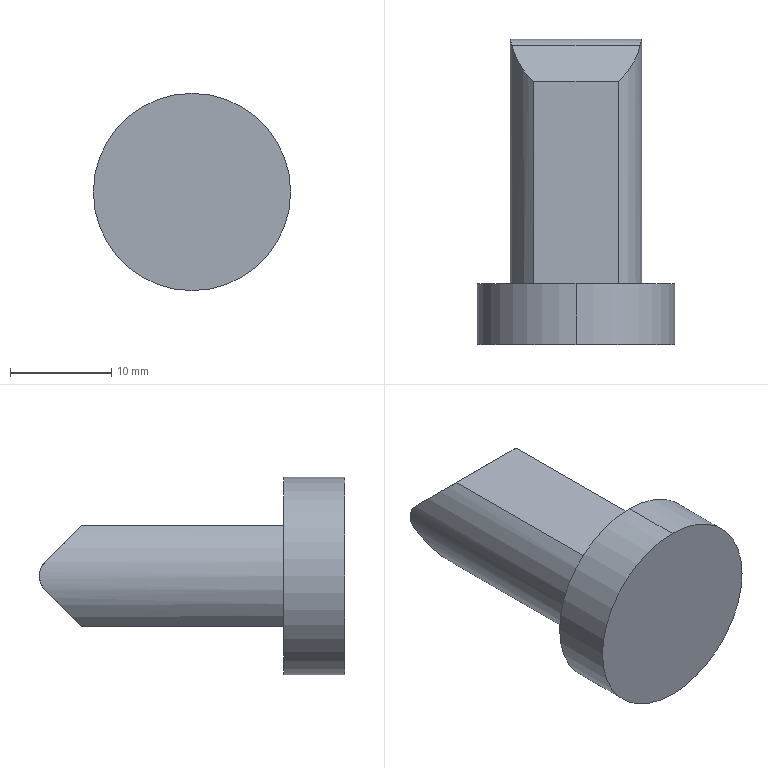Part | STEP file | Trava gavetas - Torre - 1 cav | 1 solid | 11 faces | box 19.5 x 30.172 x 19.5 mm | volume 4402 mm3 | plane 6 | cylinder 5 | commonest cylinder face diameters 13 x2 19.5 x2 4 x1
STEP:
#1=CARTESIAN_POINT('',(0.,0.,0.));
#2=DIRECTION('',(0.,0.,1.));
#3=DIRECTION('',(1.,0.,0.));
#4=AXIS2_PLACEMENT_3D('',#1,#2,#3);
#5=CARTESIAN_POINT('',(0.,0.,9.75));
#6=VERTEX_POINT('',#5);
#7=CARTESIAN_POINT('',(0.,0.,-9.75));
#8=VERTEX_POINT('',#7);
#9=CARTESIAN_POINT('',(0.,0.,0.));
#10=DIRECTION('',(0.,1.,0.));
#11=DIRECTION('',(0.,0.,1.));
#12=AXIS2_PLACEMENT_3D('',#9,#10,#11);
#13=CIRCLE('',#12,9.75);
#14=CARTESIAN_POINT('',(0.,31.,0.));
#15=DIRECTION('',(0.,1.,0.));
#16=DIRECTION('',(0.,0.,1.));
#17=AXIS2_PLACEMENT_3D('',#14,#15,#16);
#18=CYLINDRICAL_SURFACE('',#17,9.75);
#19=CARTESIAN_POINT('',(0.,-31.));
#20=DIRECTION('',(1.,0.));
#21=VECTOR('',#20,1.);
#22=LINE('',#19,#21);
#23=(GEOMETRIC_REPRESENTATION_CONTEXT(2)PARAMETRIC_REPRESENTATION_CONTEXT()REPRESENTATION_CONTEXT('',''));
#24=DEFINITIONAL_REPRESENTATION('',(#22),#23);
#25=PCURVE('',#18,#24);
#26=CARTESIAN_POINT('',(0.,0.,0.));
#27=DIRECTION('',(0.,1.,0.));
#28=DIRECTION('',(0.,0.,1.));
#29=AXIS2_PLACEMENT_3D('',#26,#27,#28);
#30=PLANE('',#29);
#31=CARTESIAN_POINT('',(0.,0.));
#32=DIRECTION('',(1.,0.));
#33=AXIS2_PLACEMENT_2D('',#31,#32);
#34=CIRCLE('',#33,9.75);
#35=(GEOMETRIC_REPRESENTATION_CONTEXT(2)PARAMETRIC_REPRESENTATION_CONTEXT()REPRESENTATION_CONTEXT('',''));
#36=DEFINITIONAL_REPRESENTATION('',(#34),#35);
#37=PCURVE('',#30,#36);
#38=SURFACE_CURVE('',#13,(#25,#37),.PCURVE_S1.);
#39=EDGE_CURVE('',#6,#8,#38,.T.);
#40=ORIENTED_EDGE('',*,*,#39,.T.);
#41=CARTESIAN_POINT('',(0.,6.,-9.75));
#42=VERTEX_POINT('',#41);
#43=CARTESIAN_POINT('',(0.,31.,-9.75));
#44=DIRECTION('',(0.,1.,0.));
#45=VECTOR('',#44,1.);
#46=LINE('',#43,#45);
#47=CARTESIAN_POINT('',(3.142,0.));
#48=DIRECTION('',(0.,1.));
#49=VECTOR('',#48,1.);
#50=LINE('',#47,#49);
#51=(GEOMETRIC_REPRESENTATION_CONTEXT(2)PARAMETRIC_REPRESENTATION_CONTEXT()REPRESENTATION_CONTEXT('',''));
#52=DEFINITIONAL_REPRESENTATION('',(#50),#51);
#53=PCURVE('',#18,#52);
#54=CARTESIAN_POINT('',(0.,31.,0.));
#55=DIRECTION('',(0.,1.,0.));
#56=DIRECTION('',(0.,0.,1.));
#57=AXIS2_PLACEMENT_3D('',#54,#55,#56);
#58=CYLINDRICAL_SURFACE('',#57,9.75);
#59=CARTESIAN_POINT('',(3.142,0.));
#60=DIRECTION('',(0.,1.));
#61=VECTOR('',#60,1.);
#62=LINE('',#59,#61);
#63=(GEOMETRIC_REPRESENTATION_CONTEXT(2)PARAMETRIC_REPRESENTATION_CONTEXT()REPRESENTATION_CONTEXT('',''));
#64=DEFINITIONAL_REPRESENTATION('',(#62),#63);
#65=PCURVE('',#58,#64);
#66=SURFACE_CURVE('',#46,(#53,#65),.PCURVE_S1.);
#67=EDGE_CURVE('',#8,#42,#66,.T.);
#68=ORIENTED_EDGE('',*,*,#67,.T.);
#69=CARTESIAN_POINT('',(0.,6.,9.75));
#70=VERTEX_POINT('',#69);
#71=CARTESIAN_POINT('',(0.,6.,0.));
#72=DIRECTION('',(0.,1.,0.));
#73=DIRECTION('',(0.,0.,1.));
#74=AXIS2_PLACEMENT_3D('',#71,#72,#73);
#75=CIRCLE('',#74,9.75);
#76=CARTESIAN_POINT('',(0.,-25.));
#77=DIRECTION('',(1.,0.));
#78=VECTOR('',#77,1.);
#79=LINE('',#76,#78);
#80=(GEOMETRIC_REPRESENTATION_CONTEXT(2)PARAMETRIC_REPRESENTATION_CONTEXT()REPRESENTATION_CONTEXT('',''));
#81=DEFINITIONAL_REPRESENTATION('',(#79),#80);
#82=PCURVE('',#18,#81);
#83=CARTESIAN_POINT('',(0.,6.,-9.75));
#84=DIRECTION('',(0.,-1.,0.));
#85=DIRECTION('',(0.,0.,-1.));
#86=AXIS2_PLACEMENT_3D('',#83,#84,#85);
#87=PLANE('',#86);
#88=CARTESIAN_POINT('',(-19.5,0.));
#89=CARTESIAN_POINT('',(-19.5,16.887));
#90=CARTESIAN_POINT('',(-4.875,8.444));
#91=CARTESIAN_POINT('',(9.75,0.));
#92=CARTESIAN_POINT('',(-4.875,-8.444));
#93=CARTESIAN_POINT('',(-19.5,-16.887));
#94=CARTESIAN_POINT('',(-19.5,0.));
#95=(BOUNDED_CURVE()B_SPLINE_CURVE(2,(#88,#89,#90,#91,#92,#93,#94),.UNSPECIFIED.,.T.,.F.)B_SPLINE_CURVE_WITH_KNOTS((1,2,2,2,2,1),(-2.094,0.,2.094,4.189,6.283,8.378),.UNSPECIFIED.)CURVE()GEOMETRIC_REPRESENTATION_ITEM()RATIONAL_B_SPLINE_CURVE((1.,0.5,1.,0.5,1.,0.5,1.))REPRESENTATION_ITEM(''));
#96=(GEOMETRIC_REPRESENTATION_CONTEXT(2)PARAMETRIC_REPRESENTATION_CONTEXT()REPRESENTATION_CONTEXT('',''));
#97=DEFINITIONAL_REPRESENTATION('',(#95),#96);
#98=PCURVE('',#87,#97);
#99=SURFACE_CURVE('',#75,(#82,#98),.PCURVE_S1.);
#100=EDGE_CURVE('',#70,#42,#99,.T.);
#101=ORIENTED_EDGE('',*,*,#100,.F.);
#102=CARTESIAN_POINT('',(0.,31.,9.75));
#103=DIRECTION('',(0.,1.,0.));
#104=VECTOR('',#103,1.);
#105=LINE('',#102,#104);
#106=CARTESIAN_POINT('',(0.,0.));
#107=DIRECTION('',(0.,1.));
#108=VECTOR('',#107,1.);
#109=LINE('',#106,#108);
#110=(GEOMETRIC_REPRESENTATION_CONTEXT(2)PARAMETRIC_REPRESENTATION_CONTEXT()REPRESENTATION_CONTEXT('',''));
#111=DEFINITIONAL_REPRESENTATION('',(#109),#110);
#112=PCURVE('',#18,#111);
#113=CARTESIAN_POINT('',(6.283,0.));
#114=DIRECTION('',(0.,1.));
#115=VECTOR('',#114,1.);
#116=LINE('',#113,#115);
#117=(GEOMETRIC_REPRESENTATION_CONTEXT(2)PARAMETRIC_REPRESENTATION_CONTEXT()REPRESENTATION_CONTEXT('',''));
#118=DEFINITIONAL_REPRESENTATION('',(#116),#117);
#119=PCURVE('',#58,#118);
#120=SURFACE_CURVE('',#105,(#112,#119),.PCURVE_S1.);
#121=EDGE_CURVE('',#6,#70,#120,.T.);
#122=ORIENTED_EDGE('',*,*,#121,.F.);
#123=EDGE_LOOP('',(#40,#68,#101,#122));
#124=FACE_BOUND('',#123,.T.);
#125=ADVANCED_FACE('',(#124),#18,.T.);
#126=CARTESIAN_POINT('',(-4.153,26.,5.));
#127=VERTEX_POINT('',#126);
#128=CARTESIAN_POINT('',(-4.153,6.,5.));
#129=VERTEX_POINT('',#128);
#130=CARTESIAN_POINT('',(-4.153,31.,5.));
#131=DIRECTION('',(0.,-1.,0.));
#132=VECTOR('',#131,1.);
#133=LINE('',#130,#132);
#134=CARTESIAN_POINT('',(0.,31.,0.));
#135=DIRECTION('',(0.,1.,0.));
#136=DIRECTION('',(0.,0.,1.));
#137=AXIS2_PLACEMENT_3D('',#134,#135,#136);
#138=CYLINDRICAL_SURFACE('',#137,6.5);
#139=CARTESIAN_POINT('',(5.59,0.));
#140=DIRECTION('',(0.,-1.));
#141=VECTOR('',#140,1.);
#142=LINE('',#139,#141);
#143=(GEOMETRIC_REPRESENTATION_CONTEXT(2)PARAMETRIC_REPRESENTATION_CONTEXT()REPRESENTATION_CONTEXT('',''));
#144=DEFINITIONAL_REPRESENTATION('',(#142),#143);
#145=PCURVE('',#138,#144);
#146=CARTESIAN_POINT('',(28.,6.,5.));
#147=DIRECTION('',(0.,0.,1.));
#148=DIRECTION('',(0.,-1.,0.));
#149=AXIS2_PLACEMENT_3D('',#146,#147,#148);
#150=PLANE('',#149);
#151=CARTESIAN_POINT('',(-25.,-32.153));
#152=DIRECTION('',(1.,0.));
#153=VECTOR('',#152,1.);
#154=LINE('',#151,#153);
#155=(GEOMETRIC_REPRESENTATION_CONTEXT(2)PARAMETRIC_REPRESENTATION_CONTEXT()REPRESENTATION_CONTEXT('',''));
#156=DEFINITIONAL_REPRESENTATION('',(#154),#155);
#157=PCURVE('',#150,#156);
#158=SURFACE_CURVE('',#133,(#145,#157),.PCURVE_S1.);
#159=EDGE_CURVE('',#127,#129,#158,.T.);
#160=ORIENTED_EDGE('',*,*,#159,.F.);
#161=CARTESIAN_POINT('',(-6.344,29.586,1.414));
#162=VERTEX_POINT('',#161);
#163=CARTESIAN_POINT('',(-6.344,29.586,1.414));
#164=CARTESIAN_POINT('',(-6.028,28.168,2.832));
#165=CARTESIAN_POINT('',(-5.271,26.928,4.072));
#166=CARTESIAN_POINT('',(-4.153,26.,5.));
#167=(BOUNDED_CURVE()B_SPLINE_CURVE(3,(#163,#164,#165,#166),.UNSPECIFIED.,.F.,.F.)B_SPLINE_CURVE_WITH_KNOTS((4,4),(1.79,2.448),.PIECEWISE_BEZIER_KNOTS.)CURVE()GEOMETRIC_REPRESENTATION_ITEM()RATIONAL_B_SPLINE_CURVE((1.,0.9642,0.9642,1.))REPRESENTATION_ITEM(''));
#168=CARTESIAN_POINT('',(4.932,-1.414));
#169=CARTESIAN_POINT('',(4.942,-1.476));
#170=CARTESIAN_POINT('',(4.961,-1.601));
#171=CARTESIAN_POINT('',(4.991,-1.786));
#172=CARTESIAN_POINT('',(5.02,-1.971));
#173=CARTESIAN_POINT('',(5.05,-2.155));
#174=CARTESIAN_POINT('',(5.08,-2.337));
#175=CARTESIAN_POINT('',(5.11,-2.518));
#176=CARTESIAN_POINT('',(5.14,-2.697));
#177=CARTESIAN_POINT('',(5.17,-2.874));
#178=CARTESIAN_POINT('',(5.2,-3.049));
#179=CARTESIAN_POINT('',(5.231,-3.221));
#180=CARTESIAN_POINT('',(5.261,-3.39));
#181=CARTESIAN_POINT('',(5.291,-3.556));
#182=CARTESIAN_POINT('',(5.321,-3.718));
#183=CARTESIAN_POINT('',(5.351,-3.877));
#184=CARTESIAN_POINT('',(5.382,-4.033));
#185=CARTESIAN_POINT('',(5.412,-4.184));
#186=CARTESIAN_POINT('',(5.442,-4.331));
#187=CARTESIAN_POINT('',(5.471,-4.474));
#188=CARTESIAN_POINT('',(5.501,-4.613));
#189=CARTESIAN_POINT('',(5.531,-4.747));
#190=CARTESIAN_POINT('',(5.561,-4.876));
#191=CARTESIAN_POINT('',(5.58,-4.959));
#192=CARTESIAN_POINT('',(5.59,-5.));
#193=B_SPLINE_CURVE_WITH_KNOTS('',3,(#168,#169,#170,#171,#172,#173,#174,#175,#176,#177,#178,#179,#180,#181,#182,#183,#184,#185,#186,#187,#188,#189,#190,#191,#192),.UNSPECIFIED.,.F.,.F.,(4,1,1,1,1,1,1,1,1,1,1,1,1,1,1,1,1,1,1,1,1,1,4),(1.79,1.82,1.85,1.88,1.91,1.94,1.97,2.,2.03,2.059,2.089,2.119,2.149,2.179,2.209,2.239,2.269,2.299,2.329,2.359,2.389,2.419,2.448),.QUASI_UNIFORM_KNOTS.);
#194=(GEOMETRIC_REPRESENTATION_CONTEXT(2)PARAMETRIC_REPRESENTATION_CONTEXT()REPRESENTATION_CONTEXT('',''));
#195=DEFINITIONAL_REPRESENTATION('',(#193),#194);
#196=PCURVE('',#138,#195);
#197=CARTESIAN_POINT('',(28.,26.,5.));
#198=DIRECTION('',(0.,0.7071,0.7071));
#199=DIRECTION('',(0.,-0.7071,0.7071));
#200=AXIS2_PLACEMENT_3D('',#197,#198,#199);
#201=PLANE('',#200);
#202=CARTESIAN_POINT('',(-5.071,-34.344));
#203=CARTESIAN_POINT('',(-3.066,-34.028));
#204=CARTESIAN_POINT('',(-1.313,-33.271));
#205=CARTESIAN_POINT('',(0.,-32.153));
#206=(BOUNDED_CURVE()B_SPLINE_CURVE(3,(#202,#203,#204,#205),.UNSPECIFIED.,.F.,.F.)B_SPLINE_CURVE_WITH_KNOTS((4,4),(1.79,2.448),.PIECEWISE_BEZIER_KNOTS.)CURVE()GEOMETRIC_REPRESENTATION_ITEM()RATIONAL_B_SPLINE_CURVE((1.,0.9642,0.9642,1.))REPRESENTATION_ITEM(''));
#207=(GEOMETRIC_REPRESENTATION_CONTEXT(2)PARAMETRIC_REPRESENTATION_CONTEXT()REPRESENTATION_CONTEXT('',''));
#208=DEFINITIONAL_REPRESENTATION('',(#206),#207);
#209=PCURVE('',#201,#208);
#210=SURFACE_CURVE('',#167,(#196,#209),.PCURVE_S1.);
#211=EDGE_CURVE('',#162,#127,#210,.T.);
#212=ORIENTED_EDGE('',*,*,#211,.F.);
#213=CARTESIAN_POINT('',(-6.344,29.586,-1.414));
#214=VERTEX_POINT('',#213);
#215=CARTESIAN_POINT('',(-6.344,29.586,-1.414));
#216=CARTESIAN_POINT('',(-6.365,29.679,-1.321));
#217=CARTESIAN_POINT('',(-6.385,29.761,-1.221));
#218=CARTESIAN_POINT('',(-6.423,29.905,-1.006));
#219=CARTESIAN_POINT('',(-6.44,29.968,-0.8891));
#220=CARTESIAN_POINT('',(-6.469,30.068,-0.6472));
#221=CARTESIAN_POINT('',(-6.48,30.107,-0.5225));
#222=CARTESIAN_POINT('',(-6.496,30.158,-0.2654));
#223=CARTESIAN_POINT('',(-6.5,30.172,-0.1321));
#224=CARTESIAN_POINT('',(-6.5,30.172,0.2613));
#225=CARTESIAN_POINT('',(-6.483,30.119,0.5256));
#226=CARTESIAN_POINT('',(-6.44,29.969,0.8868));
#227=CARTESIAN_POINT('',(-6.423,29.907,1.003));
#228=CARTESIAN_POINT('',(-6.385,29.761,1.221));
#229=CARTESIAN_POINT('',(-6.365,29.679,1.321));
#230=CARTESIAN_POINT('',(-6.344,29.586,1.414));
#231=B_SPLINE_CURVE_WITH_KNOTS('',3,(#215,#216,#217,#218,#219,#220,#221,#222,#223,#224,#225,#226,#227,#228,#229,#230),.UNSPECIFIED.,.F.,.F.,(4,2,2,2,2,2,2,4),(0.,0.000393,0.0007859,0.001179,0.001572,0.002358,0.002751,0.003144),.UNSPECIFIED.);
#232=CARTESIAN_POINT('',(4.493,-1.414));
#233=CARTESIAN_POINT('',(4.496,-1.397));
#234=CARTESIAN_POINT('',(4.501,-1.364));
#235=CARTESIAN_POINT('',(4.509,-1.317));
#236=CARTESIAN_POINT('',(4.518,-1.271));
#237=CARTESIAN_POINT('',(4.527,-1.228));
#238=CARTESIAN_POINT('',(4.536,-1.187));
#239=CARTESIAN_POINT('',(4.545,-1.147));
#240=CARTESIAN_POINT('',(4.554,-1.11));
#241=CARTESIAN_POINT('',(4.564,-1.074));
#242=CARTESIAN_POINT('',(4.574,-1.041));
#243=CARTESIAN_POINT('',(4.584,-1.01));
#244=CARTESIAN_POINT('',(4.594,-0.9814));
#245=CARTESIAN_POINT('',(4.604,-0.9552));
#246=CARTESIAN_POINT('',(4.615,-0.9314));
#247=CARTESIAN_POINT('',(4.625,-0.91));
#248=CARTESIAN_POINT('',(4.636,-0.8911));
#249=CARTESIAN_POINT('',(4.646,-0.8746));
#250=CARTESIAN_POINT('',(4.657,-0.8605));
#251=CARTESIAN_POINT('',(4.668,-0.8489));
#252=CARTESIAN_POINT('',(4.679,-0.8398));
#253=CARTESIAN_POINT('',(4.69,-0.8333));
#254=CARTESIAN_POINT('',(4.701,-0.8293));
#255=CARTESIAN_POINT('',(4.712,-0.828));
#256=CARTESIAN_POINT('',(4.723,-0.8293));
#257=CARTESIAN_POINT('',(4.734,-0.8332));
#258=CARTESIAN_POINT('',(4.745,-0.8396));
#259=CARTESIAN_POINT('',(4.756,-0.8486));
#260=CARTESIAN_POINT('',(4.767,-0.8601));
#261=CARTESIAN_POINT('',(4.778,-0.8742));
#262=CARTESIAN_POINT('',(4.789,-0.8907));
#263=CARTESIAN_POINT('',(4.799,-0.9096));
#264=CARTESIAN_POINT('',(4.81,-0.9309));
#265=CARTESIAN_POINT('',(4.82,-0.9546));
#266=CARTESIAN_POINT('',(4.831,-0.9807));
#267=CARTESIAN_POINT('',(4.841,-1.009));
#268=CARTESIAN_POINT('',(4.851,-1.04));
#269=CARTESIAN_POINT('',(4.861,-1.073));
#270=CARTESIAN_POINT('',(4.87,-1.109));
#271=CARTESIAN_POINT('',(4.88,-1.146));
#272=CARTESIAN_POINT('',(4.889,-1.186));
#273=CARTESIAN_POINT('',(4.898,-1.227));
#274=CARTESIAN_POINT('',(4.907,-1.271));
#275=CARTESIAN_POINT('',(4.915,-1.317));
#276=CARTESIAN_POINT('',(4.924,-1.364));
#277=CARTESIAN_POINT('',(4.929,-1.397));
#278=CARTESIAN_POINT('',(4.932,-1.414));
#279=B_SPLINE_CURVE_WITH_KNOTS('',3,(#232,#233,#234,#235,#236,#237,#238,#239,#240,#241,#242,#243,#244,#245,#246,#247,#248,#249,#250,#251,#252,#253,#254,#255,#256,#257,#258,#259,#260,#261,#262,#263,#264,#265,#266,#267,#268,#269,#270,#271,#272,#273,#274,#275,#276,#277,#278),.UNSPECIFIED.,.F.,.F.,(4,1,1,1,1,1,1,1,1,1,1,1,1,1,1,1,1,1,1,1,1,1,1,1,1,1,1,1,1,1,1,1,1,1,1,1,1,1,1,1,1,1,1,1,4),(0.,0.00007145,0.0001429,0.0002143,0.0002858,0.0003572,0.0004287,0.0005001,0.0005716,0.000643,0.0007145,0.0007859,0.0008574,0.0009288,0.001,0.001072,0.001143,0.001215,0.001286,0.001358,0.001429,0.0015,0.001572,0.001643,0.001715,0.001786,0.001858,0.001929,0.002001,0.002072,0.002143,0.002215,0.002286,0.002358,0.002429,0.002501,0.002572,0.002644,0.002715,0.002786,0.002858,0.002929,0.003001,0.003072,0.003144),.QUASI_UNIFORM_KNOTS.);
#280=(GEOMETRIC_REPRESENTATION_CONTEXT(2)PARAMETRIC_REPRESENTATION_CONTEXT()REPRESENTATION_CONTEXT('',''));
#281=DEFINITIONAL_REPRESENTATION('',(#279),#280);
#282=PCURVE('',#138,#281);
#283=CARTESIAN_POINT('',(28.,28.172,0.));
#284=DIRECTION('',(-1.,0.,0.));
#285=DIRECTION('',(0.,0.,1.));
#286=AXIS2_PLACEMENT_3D('',#283,#284,#285);
#287=CYLINDRICAL_SURFACE('',#286,2.);
#288=CARTESIAN_POINT('',(2.356,34.344));
#289=CARTESIAN_POINT('',(2.344,34.348));
#290=CARTESIAN_POINT('',(2.32,34.356));
#291=CARTESIAN_POINT('',(2.285,34.367));
#292=CARTESIAN_POINT('',(2.25,34.378));
#293=CARTESIAN_POINT('',(2.214,34.388));
#294=CARTESIAN_POINT('',(2.179,34.399));
#295=CARTESIAN_POINT('',(2.144,34.409));
#296=CARTESIAN_POINT('',(2.108,34.419));
#297=CARTESIAN_POINT('',(2.072,34.429));
#298=CARTESIAN_POINT('',(2.037,34.438));
#299=CARTESIAN_POINT('',(2.001,34.446));
#300=CARTESIAN_POINT('',(1.965,34.455));
#301=CARTESIAN_POINT('',(1.929,34.462));
#302=CARTESIAN_POINT('',(1.894,34.469));
#303=CARTESIAN_POINT('',(1.858,34.475));
#304=CARTESIAN_POINT('',(1.823,34.481));
#305=CARTESIAN_POINT('',(1.787,34.486));
#306=CARTESIAN_POINT('',(1.751,34.49));
#307=CARTESIAN_POINT('',(1.715,34.494));
#308=CARTESIAN_POINT('',(1.679,34.497));
#309=CARTESIAN_POINT('',(1.643,34.499));
#310=CARTESIAN_POINT('',(1.607,34.5));
#311=CARTESIAN_POINT('',(1.571,34.5));
#312=CARTESIAN_POINT('',(1.536,34.5));
#313=CARTESIAN_POINT('',(1.5,34.499));
#314=CARTESIAN_POINT('',(1.464,34.497));
#315=CARTESIAN_POINT('',(1.428,34.494));
#316=CARTESIAN_POINT('',(1.392,34.49));
#317=CARTESIAN_POINT('',(1.356,34.486));
#318=CARTESIAN_POINT('',(1.32,34.481));
#319=CARTESIAN_POINT('',(1.285,34.475));
#320=CARTESIAN_POINT('',(1.249,34.469));
#321=CARTESIAN_POINT('',(1.213,34.462));
#322=CARTESIAN_POINT('',(1.178,34.455));
#323=CARTESIAN_POINT('',(1.142,34.447));
#324=CARTESIAN_POINT('',(1.106,34.438));
#325=CARTESIAN_POINT('',(1.071,34.429));
#326=CARTESIAN_POINT('',(1.035,34.419));
#327=CARTESIAN_POINT('',(0.9991,34.409));
#328=CARTESIAN_POINT('',(0.9634,34.399));
#329=CARTESIAN_POINT('',(0.9278,34.388));
#330=CARTESIAN_POINT('',(0.8923,34.378));
#331=CARTESIAN_POINT('',(0.8567,34.367));
#332=CARTESIAN_POINT('',(0.8211,34.356));
#333=CARTESIAN_POINT('',(0.7973,34.348));
#334=CARTESIAN_POINT('',(0.7854,34.344));
#335=B_SPLINE_CURVE_WITH_KNOTS('',3,(#288,#289,#290,#291,#292,#293,#294,#295,#296,#297,#298,#299,#300,#301,#302,#303,#304,#305,#306,#307,#308,#309,#310,#311,#312,#313,#314,#315,#316,#317,#318,#319,#320,#321,#322,#323,#324,#325,#326,#327,#328,#329,#330,#331,#332,#333,#334),.UNSPECIFIED.,.F.,.F.,(4,1,1,1,1,1,1,1,1,1,1,1,1,1,1,1,1,1,1,1,1,1,1,1,1,1,1,1,1,1,1,1,1,1,1,1,1,1,1,1,1,1,1,1,4),(0.,0.00007145,0.0001429,0.0002143,0.0002858,0.0003572,0.0004287,0.0005001,0.0005716,0.000643,0.0007145,0.0007859,0.0008574,0.0009288,0.001,0.001072,0.001143,0.001215,0.001286,0.001358,0.001429,0.0015,0.001572,0.001643,0.001715,0.001786,0.001858,0.001929,0.002001,0.002072,0.002143,0.002215,0.002286,0.002358,0.002429,0.002501,0.002572,0.002644,0.002715,0.002786,0.002858,0.002929,0.003001,0.003072,0.003144),.QUASI_UNIFORM_KNOTS.);
#336=(GEOMETRIC_REPRESENTATION_CONTEXT(2)PARAMETRIC_REPRESENTATION_CONTEXT()REPRESENTATION_CONTEXT('',''));
#337=DEFINITIONAL_REPRESENTATION('',(#335),#336);
#338=PCURVE('',#287,#337);
#339=SURFACE_CURVE('',#231,(#282,#338),.PCURVE_S1.);
#340=EDGE_CURVE('',#214,#162,#339,.T.);
#341=ORIENTED_EDGE('',*,*,#340,.F.);
#342=CARTESIAN_POINT('',(-4.153,26.,-5.));
#343=VERTEX_POINT('',#342);
#344=CARTESIAN_POINT('',(-4.153,26.,-5.));
#345=CARTESIAN_POINT('',(-5.271,26.928,-4.072));
#346=CARTESIAN_POINT('',(-6.028,28.168,-2.832));
#347=CARTESIAN_POINT('',(-6.344,29.586,-1.414));
#348=(BOUNDED_CURVE()B_SPLINE_CURVE(3,(#344,#345,#346,#347),.UNSPECIFIED.,.F.,.F.)B_SPLINE_CURVE_WITH_KNOTS((4,4),(3.835,4.493),.PIECEWISE_BEZIER_KNOTS.)CURVE()GEOMETRIC_REPRESENTATION_ITEM()RATIONAL_B_SPLINE_CURVE((1.,0.9642,0.9642,1.))REPRESENTATION_ITEM(''));
#349=CARTESIAN_POINT('',(3.835,-5.));
#350=CARTESIAN_POINT('',(3.845,-4.959));
#351=CARTESIAN_POINT('',(3.864,-4.876));
#352=CARTESIAN_POINT('',(3.894,-4.747));
#353=CARTESIAN_POINT('',(3.923,-4.613));
#354=CARTESIAN_POINT('',(3.953,-4.474));
#355=CARTESIAN_POINT('',(3.983,-4.331));
#356=CARTESIAN_POINT('',(4.013,-4.184));
#357=CARTESIAN_POINT('',(4.043,-4.033));
#358=CARTESIAN_POINT('',(4.073,-3.877));
#359=CARTESIAN_POINT('',(4.104,-3.718));
#360=CARTESIAN_POINT('',(4.134,-3.556));
#361=CARTESIAN_POINT('',(4.164,-3.39));
#362=CARTESIAN_POINT('',(4.194,-3.221));
#363=CARTESIAN_POINT('',(4.224,-3.049));
#364=CARTESIAN_POINT('',(4.254,-2.874));
#365=CARTESIAN_POINT('',(4.285,-2.697));
#366=CARTESIAN_POINT('',(4.315,-2.518));
#367=CARTESIAN_POINT('',(4.345,-2.337));
#368=CARTESIAN_POINT('',(4.375,-2.155));
#369=CARTESIAN_POINT('',(4.404,-1.971));
#370=CARTESIAN_POINT('',(4.434,-1.786));
#371=CARTESIAN_POINT('',(4.464,-1.601));
#372=CARTESIAN_POINT('',(4.483,-1.476));
#373=CARTESIAN_POINT('',(4.493,-1.414));
#374=B_SPLINE_CURVE_WITH_KNOTS('',3,(#349,#350,#351,#352,#353,#354,#355,#356,#357,#358,#359,#360,#361,#362,#363,#364,#365,#366,#367,#368,#369,#370,#371,#372,#373),.UNSPECIFIED.,.F.,.F.,(4,1,1,1,1,1,1,1,1,1,1,1,1,1,1,1,1,1,1,1,1,1,4),(3.835,3.865,3.895,3.925,3.954,3.984,4.014,4.044,4.074,4.104,4.134,4.164,4.194,4.224,4.254,4.284,4.314,4.343,4.373,4.403,4.433,4.463,4.493),.QUASI_UNIFORM_KNOTS.);
#375=(GEOMETRIC_REPRESENTATION_CONTEXT(2)PARAMETRIC_REPRESENTATION_CONTEXT()REPRESENTATION_CONTEXT('',''));
#376=DEFINITIONAL_REPRESENTATION('',(#374),#375);
#377=PCURVE('',#138,#376);
#378=CARTESIAN_POINT('',(28.,26.,-5.));
#379=DIRECTION('',(0.,0.7071,-0.7071));
#380=DIRECTION('',(0.,0.7071,0.7071));
#381=AXIS2_PLACEMENT_3D('',#378,#379,#380);
#382=PLANE('',#381);
#383=CARTESIAN_POINT('',(0.,-32.153));
#384=CARTESIAN_POINT('',(1.313,-33.271));
#385=CARTESIAN_POINT('',(3.066,-34.028));
#386=CARTESIAN_POINT('',(5.071,-34.344));
#387=(BOUNDED_CURVE()B_SPLINE_CURVE(3,(#383,#384,#385,#386),.UNSPECIFIED.,.F.,.F.)B_SPLINE_CURVE_WITH_KNOTS((4,4),(3.835,4.493),.PIECEWISE_BEZIER_KNOTS.)CURVE()GEOMETRIC_REPRESENTATION_ITEM()RATIONAL_B_SPLINE_CURVE((1.,0.9642,0.9642,1.))REPRESENTATION_ITEM(''));
#388=(GEOMETRIC_REPRESENTATION_CONTEXT(2)PARAMETRIC_REPRESENTATION_CONTEXT()REPRESENTATION_CONTEXT('',''));
#389=DEFINITIONAL_REPRESENTATION('',(#387),#388);
#390=PCURVE('',#382,#389);
#391=SURFACE_CURVE('',#348,(#377,#390),.PCURVE_S1.);
#392=EDGE_CURVE('',#343,#214,#391,.T.);
#393=ORIENTED_EDGE('',*,*,#392,.F.);
#394=CARTESIAN_POINT('',(-4.153,6.,-5.));
#395=VERTEX_POINT('',#394);
#396=CARTESIAN_POINT('',(-4.153,31.,-5.));
#397=DIRECTION('',(0.,1.,0.));
#398=VECTOR('',#397,1.);
#399=LINE('',#396,#398);
#400=CARTESIAN_POINT('',(3.835,0.));
#401=DIRECTION('',(0.,1.));
#402=VECTOR('',#401,1.);
#403=LINE('',#400,#402);
#404=(GEOMETRIC_REPRESENTATION_CONTEXT(2)PARAMETRIC_REPRESENTATION_CONTEXT()REPRESENTATION_CONTEXT('',''));
#405=DEFINITIONAL_REPRESENTATION('',(#403),#404);
#406=PCURVE('',#138,#405);
#407=CARTESIAN_POINT('',(28.,6.,-5.));
#408=DIRECTION('',(0.,0.,-1.));
#409=DIRECTION('',(0.,1.,0.));
#410=AXIS2_PLACEMENT_3D('',#407,#408,#409);
#411=PLANE('',#410);
#412=CARTESIAN_POINT('',(25.,-32.153));
#413=DIRECTION('',(1.,0.));
#414=VECTOR('',#413,1.);
#415=LINE('',#412,#414);
#416=(GEOMETRIC_REPRESENTATION_CONTEXT(2)PARAMETRIC_REPRESENTATION_CONTEXT()REPRESENTATION_CONTEXT('',''));
#417=DEFINITIONAL_REPRESENTATION('',(#415),#416);
#418=PCURVE('',#411,#417);
#419=SURFACE_CURVE('',#399,(#406,#418),.PCURVE_S1.);
#420=EDGE_CURVE('',#395,#343,#419,.T.);
#421=ORIENTED_EDGE('',*,*,#420,.F.);
#422=CARTESIAN_POINT('',(0.,6.,0.));
#423=DIRECTION('',(0.,1.,0.));
#424=DIRECTION('',(0.,0.,1.));
#425=AXIS2_PLACEMENT_3D('',#422,#423,#424);
#426=CIRCLE('',#425,6.5);
#427=CARTESIAN_POINT('',(0.,-25.));
#428=DIRECTION('',(1.,0.));
#429=VECTOR('',#428,1.);
#430=LINE('',#427,#429);
#431=(GEOMETRIC_REPRESENTATION_CONTEXT(2)PARAMETRIC_REPRESENTATION_CONTEXT()REPRESENTATION_CONTEXT('',''));
#432=DEFINITIONAL_REPRESENTATION('',(#430),#431);
#433=PCURVE('',#138,#432);
#434=CARTESIAN_POINT('',(-16.25,0.));
#435=CARTESIAN_POINT('',(-16.25,11.258));
#436=CARTESIAN_POINT('',(-6.5,5.629));
#437=CARTESIAN_POINT('',(3.25,0.));
#438=CARTESIAN_POINT('',(-6.5,-5.629));
#439=CARTESIAN_POINT('',(-16.25,-11.258));
#440=CARTESIAN_POINT('',(-16.25,0.));
#441=(BOUNDED_CURVE()B_SPLINE_CURVE(2,(#434,#435,#436,#437,#438,#439,#440),.UNSPECIFIED.,.T.,.F.)B_SPLINE_CURVE_WITH_KNOTS((1,2,2,2,2,1),(-2.094,0.,2.094,4.189,6.283,8.378),.UNSPECIFIED.)CURVE()GEOMETRIC_REPRESENTATION_ITEM()RATIONAL_B_SPLINE_CURVE((1.,0.5,1.,0.5,1.,0.5,1.))REPRESENTATION_ITEM(''));
#442=(GEOMETRIC_REPRESENTATION_CONTEXT(2)PARAMETRIC_REPRESENTATION_CONTEXT()REPRESENTATION_CONTEXT('',''));
#443=DEFINITIONAL_REPRESENTATION('',(#441),#442);
#444=PCURVE('',#87,#443);
#445=SURFACE_CURVE('',#426,(#433,#444),.PCURVE_S1.);
#446=EDGE_CURVE('',#395,#129,#445,.T.);
#447=ORIENTED_EDGE('',*,*,#446,.T.);
#448=EDGE_LOOP('',(#160,#212,#341,#393,#421,#447));
#449=FACE_BOUND('',#448,.T.);
#450=ADVANCED_FACE('',(#449),#138,.T.);
#451=CARTESIAN_POINT('',(4.153,6.,5.));
#452=VERTEX_POINT('',#451);
#453=CARTESIAN_POINT('',(4.153,26.,5.));
#454=VERTEX_POINT('',#453);
#455=CARTESIAN_POINT('',(4.153,31.,5.));
#456=DIRECTION('',(0.,1.,0.));
#457=VECTOR('',#456,1.);
#458=LINE('',#455,#457);
#459=CARTESIAN_POINT('',(0.,31.,0.));
#460=DIRECTION('',(0.,1.,0.));
#461=DIRECTION('',(0.,0.,1.));
#462=AXIS2_PLACEMENT_3D('',#459,#460,#461);
#463=CYLINDRICAL_SURFACE('',#462,6.5);
#464=CARTESIAN_POINT('',(0.6932,0.));
#465=DIRECTION('',(0.,1.));
#466=VECTOR('',#465,1.);
#467=LINE('',#464,#466);
#468=(GEOMETRIC_REPRESENTATION_CONTEXT(2)PARAMETRIC_REPRESENTATION_CONTEXT()REPRESENTATION_CONTEXT('',''));
#469=DEFINITIONAL_REPRESENTATION('',(#467),#468);
#470=PCURVE('',#463,#469);
#471=CARTESIAN_POINT('',(-25.,-23.847));
#472=DIRECTION('',(-1.,0.));
#473=VECTOR('',#472,1.);
#474=LINE('',#471,#473);
#475=(GEOMETRIC_REPRESENTATION_CONTEXT(2)PARAMETRIC_REPRESENTATION_CONTEXT()REPRESENTATION_CONTEXT('',''));
#476=DEFINITIONAL_REPRESENTATION('',(#474),#475);
#477=PCURVE('',#150,#476);
#478=SURFACE_CURVE('',#458,(#470,#477),.PCURVE_S1.);
#479=EDGE_CURVE('',#452,#454,#478,.T.);
#480=ORIENTED_EDGE('',*,*,#479,.F.);
#481=CARTESIAN_POINT('',(4.153,6.,-5.));
#482=VERTEX_POINT('',#481);
#483=CARTESIAN_POINT('',(0.,6.,0.));
#484=DIRECTION('',(0.,1.,0.));
#485=DIRECTION('',(0.,0.,1.));
#486=AXIS2_PLACEMENT_3D('',#483,#484,#485);
#487=CIRCLE('',#486,6.5);
#488=CARTESIAN_POINT('',(0.,-25.));
#489=DIRECTION('',(1.,0.));
#490=VECTOR('',#489,1.);
#491=LINE('',#488,#490);
#492=(GEOMETRIC_REPRESENTATION_CONTEXT(2)PARAMETRIC_REPRESENTATION_CONTEXT()REPRESENTATION_CONTEXT('',''));
#493=DEFINITIONAL_REPRESENTATION('',(#491),#492);
#494=PCURVE('',#463,#493);
#495=CARTESIAN_POINT('',(-16.25,0.));
#496=CARTESIAN_POINT('',(-16.25,11.258));
#497=CARTESIAN_POINT('',(-6.5,5.629));
#498=CARTESIAN_POINT('',(3.25,0.));
#499=CARTESIAN_POINT('',(-6.5,-5.629));
#500=CARTESIAN_POINT('',(-16.25,-11.258));
#501=CARTESIAN_POINT('',(-16.25,0.));
#502=(BOUNDED_CURVE()B_SPLINE_CURVE(2,(#495,#496,#497,#498,#499,#500,#501),.UNSPECIFIED.,.T.,.F.)B_SPLINE_CURVE_WITH_KNOTS((1,2,2,2,2,1),(-2.094,0.,2.094,4.189,6.283,8.378),.UNSPECIFIED.)CURVE()GEOMETRIC_REPRESENTATION_ITEM()RATIONAL_B_SPLINE_CURVE((1.,0.5,1.,0.5,1.,0.5,1.))REPRESENTATION_ITEM(''));
#503=(GEOMETRIC_REPRESENTATION_CONTEXT(2)PARAMETRIC_REPRESENTATION_CONTEXT()REPRESENTATION_CONTEXT('',''));
#504=DEFINITIONAL_REPRESENTATION('',(#502),#503);
#505=PCURVE('',#87,#504);
#506=SURFACE_CURVE('',#487,(#494,#505),.PCURVE_S1.);
#507=EDGE_CURVE('',#452,#482,#506,.T.);
#508=ORIENTED_EDGE('',*,*,#507,.T.);
#509=CARTESIAN_POINT('',(4.153,26.,-5.));
#510=VERTEX_POINT('',#509);
#511=CARTESIAN_POINT('',(4.153,31.,-5.));
#512=DIRECTION('',(0.,-1.,0.));
#513=VECTOR('',#512,1.);
#514=LINE('',#511,#513);
#515=CARTESIAN_POINT('',(2.448,0.));
#516=DIRECTION('',(0.,-1.));
#517=VECTOR('',#516,1.);
#518=LINE('',#515,#517);
#519=(GEOMETRIC_REPRESENTATION_CONTEXT(2)PARAMETRIC_REPRESENTATION_CONTEXT()REPRESENTATION_CONTEXT('',''));
#520=DEFINITIONAL_REPRESENTATION('',(#518),#519);
#521=PCURVE('',#463,#520);
#522=CARTESIAN_POINT('',(25.,-23.847));
#523=DIRECTION('',(-1.,0.));
#524=VECTOR('',#523,1.);
#525=LINE('',#522,#524);
#526=(GEOMETRIC_REPRESENTATION_CONTEXT(2)PARAMETRIC_REPRESENTATION_CONTEXT()REPRESENTATION_CONTEXT('',''));
#527=DEFINITIONAL_REPRESENTATION('',(#525),#526);
#528=PCURVE('',#411,#527);
#529=SURFACE_CURVE('',#514,(#521,#528),.PCURVE_S1.);
#530=EDGE_CURVE('',#510,#482,#529,.T.);
#531=ORIENTED_EDGE('',*,*,#530,.F.);
#532=CARTESIAN_POINT('',(6.344,29.586,-1.414));
#533=VERTEX_POINT('',#532);
#534=CARTESIAN_POINT('',(6.344,29.586,-1.414));
#535=CARTESIAN_POINT('',(6.028,28.168,-2.832));
#536=CARTESIAN_POINT('',(5.271,26.928,-4.072));
#537=CARTESIAN_POINT('',(4.153,26.,-5.));
#538=(BOUNDED_CURVE()B_SPLINE_CURVE(3,(#534,#535,#536,#537),.UNSPECIFIED.,.F.,.F.)B_SPLINE_CURVE_WITH_KNOTS((4,4),(1.79,2.448),.PIECEWISE_BEZIER_KNOTS.)CURVE()GEOMETRIC_REPRESENTATION_ITEM()RATIONAL_B_SPLINE_CURVE((1.,0.9642,0.9642,1.))REPRESENTATION_ITEM(''));
#539=CARTESIAN_POINT('',(1.79,-1.414));
#540=CARTESIAN_POINT('',(1.8,-1.476));
#541=CARTESIAN_POINT('',(1.82,-1.601));
#542=CARTESIAN_POINT('',(1.849,-1.786));
#543=CARTESIAN_POINT('',(1.879,-1.971));
#544=CARTESIAN_POINT('',(1.909,-2.155));
#545=CARTESIAN_POINT('',(1.939,-2.337));
#546=CARTESIAN_POINT('',(1.969,-2.518));
#547=CARTESIAN_POINT('',(1.999,-2.697));
#548=CARTESIAN_POINT('',(2.029,-2.874));
#549=CARTESIAN_POINT('',(2.059,-3.049));
#550=CARTESIAN_POINT('',(2.089,-3.221));
#551=CARTESIAN_POINT('',(2.119,-3.39));
#552=CARTESIAN_POINT('',(2.149,-3.556));
#553=CARTESIAN_POINT('',(2.18,-3.718));
#554=CARTESIAN_POINT('',(2.21,-3.877));
#555=CARTESIAN_POINT('',(2.24,-4.033));
#556=CARTESIAN_POINT('',(2.27,-4.184));
#557=CARTESIAN_POINT('',(2.3,-4.331));
#558=CARTESIAN_POINT('',(2.33,-4.474));
#559=CARTESIAN_POINT('',(2.36,-4.613));
#560=CARTESIAN_POINT('',(2.389,-4.747));
#561=CARTESIAN_POINT('',(2.419,-4.876));
#562=CARTESIAN_POINT('',(2.439,-4.959));
#563=CARTESIAN_POINT('',(2.448,-5.));
#564=B_SPLINE_CURVE_WITH_KNOTS('',3,(#539,#540,#541,#542,#543,#544,#545,#546,#547,#548,#549,#550,#551,#552,#553,#554,#555,#556,#557,#558,#559,#560,#561,#562,#563),.UNSPECIFIED.,.F.,.F.,(4,1,1,1,1,1,1,1,1,1,1,1,1,1,1,1,1,1,1,1,1,1,4),(1.79,1.82,1.85,1.88,1.91,1.94,1.97,2.,2.03,2.059,2.089,2.119,2.149,2.179,2.209,2.239,2.269,2.299,2.329,2.359,2.389,2.419,2.448),.QUASI_UNIFORM_KNOTS.);
#565=(GEOMETRIC_REPRESENTATION_CONTEXT(2)PARAMETRIC_REPRESENTATION_CONTEXT()REPRESENTATION_CONTEXT('',''));
#566=DEFINITIONAL_REPRESENTATION('',(#564),#565);
#567=PCURVE('',#463,#566);
#568=CARTESIAN_POINT('',(5.071,-21.656));
#569=CARTESIAN_POINT('',(3.066,-21.972));
#570=CARTESIAN_POINT('',(1.313,-22.729));
#571=CARTESIAN_POINT('',(0.,-23.847));
#572=(BOUNDED_CURVE()B_SPLINE_CURVE(3,(#568,#569,#570,#571),.UNSPECIFIED.,.F.,.F.)B_SPLINE_CURVE_WITH_KNOTS((4,4),(1.79,2.448),.PIECEWISE_BEZIER_KNOTS.)CURVE()GEOMETRIC_REPRESENTATION_ITEM()RATIONAL_B_SPLINE_CURVE((1.,0.9642,0.9642,1.))REPRESENTATION_ITEM(''));
#573=(GEOMETRIC_REPRESENTATION_CONTEXT(2)PARAMETRIC_REPRESENTATION_CONTEXT()REPRESENTATION_CONTEXT('',''));
#574=DEFINITIONAL_REPRESENTATION('',(#572),#573);
#575=PCURVE('',#382,#574);
#576=SURFACE_CURVE('',#538,(#567,#575),.PCURVE_S1.);
#577=EDGE_CURVE('',#533,#510,#576,.T.);
#578=ORIENTED_EDGE('',*,*,#577,.F.);
#579=CARTESIAN_POINT('',(6.344,29.586,1.414));
#580=VERTEX_POINT('',#579);
#581=CARTESIAN_POINT('',(6.344,29.586,1.414));
#582=CARTESIAN_POINT('',(6.365,29.679,1.321));
#583=CARTESIAN_POINT('',(6.385,29.761,1.221));
#584=CARTESIAN_POINT('',(6.423,29.905,1.006));
#585=CARTESIAN_POINT('',(6.44,29.968,0.8891));
#586=CARTESIAN_POINT('',(6.469,30.068,0.6472));
#587=CARTESIAN_POINT('',(6.48,30.107,0.5225));
#588=CARTESIAN_POINT('',(6.496,30.158,0.2654));
#589=CARTESIAN_POINT('',(6.5,30.172,0.1321));
#590=CARTESIAN_POINT('',(6.5,30.172,-0.2613));
#591=CARTESIAN_POINT('',(6.483,30.119,-0.5256));
#592=CARTESIAN_POINT('',(6.44,29.969,-0.8868));
#593=CARTESIAN_POINT('',(6.423,29.907,-1.003));
#594=CARTESIAN_POINT('',(6.385,29.761,-1.221));
#595=CARTESIAN_POINT('',(6.365,29.679,-1.321));
#596=CARTESIAN_POINT('',(6.344,29.586,-1.414));
#597=B_SPLINE_CURVE_WITH_KNOTS('',3,(#581,#582,#583,#584,#585,#586,#587,#588,#589,#590,#591,#592,#593,#594,#595,#596),.UNSPECIFIED.,.F.,.F.,(4,2,2,2,2,2,2,4),(0.,0.000393,0.0007859,0.001179,0.001572,0.002358,0.002751,0.003144),.UNSPECIFIED.);
#598=CARTESIAN_POINT('',(1.351,-1.414));
#599=CARTESIAN_POINT('',(1.354,-1.397));
#600=CARTESIAN_POINT('',(1.36,-1.364));
#601=CARTESIAN_POINT('',(1.368,-1.317));
#602=CARTESIAN_POINT('',(1.376,-1.271));
#603=CARTESIAN_POINT('',(1.385,-1.228));
#604=CARTESIAN_POINT('',(1.394,-1.187));
#605=CARTESIAN_POINT('',(1.403,-1.147));
#606=CARTESIAN_POINT('',(1.413,-1.11));
#607=CARTESIAN_POINT('',(1.422,-1.074));
#608=CARTESIAN_POINT('',(1.432,-1.041));
#609=CARTESIAN_POINT('',(1.442,-1.01));
#610=CARTESIAN_POINT('',(1.452,-0.9814));
#611=CARTESIAN_POINT('',(1.463,-0.9552));
#612=CARTESIAN_POINT('',(1.473,-0.9314));
#613=CARTESIAN_POINT('',(1.483,-0.91));
#614=CARTESIAN_POINT('',(1.494,-0.8911));
#615=CARTESIAN_POINT('',(1.505,-0.8746));
#616=CARTESIAN_POINT('',(1.516,-0.8605));
#617=CARTESIAN_POINT('',(1.526,-0.8489));
#618=CARTESIAN_POINT('',(1.537,-0.8398));
#619=CARTESIAN_POINT('',(1.549,-0.8333));
#620=CARTESIAN_POINT('',(1.56,-0.8293));
#621=CARTESIAN_POINT('',(1.571,-0.828));
#622=CARTESIAN_POINT('',(1.582,-0.8293));
#623=CARTESIAN_POINT('',(1.593,-0.8332));
#624=CARTESIAN_POINT('',(1.604,-0.8396));
#625=CARTESIAN_POINT('',(1.615,-0.8486));
#626=CARTESIAN_POINT('',(1.626,-0.8601));
#627=CARTESIAN_POINT('',(1.636,-0.8742));
#628=CARTESIAN_POINT('',(1.647,-0.8907));
#629=CARTESIAN_POINT('',(1.658,-0.9096));
#630=CARTESIAN_POINT('',(1.668,-0.9309));
#631=CARTESIAN_POINT('',(1.679,-0.9546));
#632=CARTESIAN_POINT('',(1.689,-0.9807));
#633=CARTESIAN_POINT('',(1.699,-1.009));
#634=CARTESIAN_POINT('',(1.709,-1.04));
#635=CARTESIAN_POINT('',(1.719,-1.073));
#636=CARTESIAN_POINT('',(1.729,-1.109));
#637=CARTESIAN_POINT('',(1.738,-1.146));
#638=CARTESIAN_POINT('',(1.747,-1.186));
#639=CARTESIAN_POINT('',(1.756,-1.227));
#640=CARTESIAN_POINT('',(1.765,-1.271));
#641=CARTESIAN_POINT('',(1.774,-1.317));
#642=CARTESIAN_POINT('',(1.782,-1.364));
#643=CARTESIAN_POINT('',(1.787,-1.397));
#644=CARTESIAN_POINT('',(1.79,-1.414));
#645=B_SPLINE_CURVE_WITH_KNOTS('',3,(#598,#599,#600,#601,#602,#603,#604,#605,#606,#607,#608,#609,#610,#611,#612,#613,#614,#615,#616,#617,#618,#619,#620,#621,#622,#623,#624,#625,#626,#627,#628,#629,#630,#631,#632,#633,#634,#635,#636,#637,#638,#639,#640,#641,#642,#643,#644),.UNSPECIFIED.,.F.,.F.,(4,1,1,1,1,1,1,1,1,1,1,1,1,1,1,1,1,1,1,1,1,1,1,1,1,1,1,1,1,1,1,1,1,1,1,1,1,1,1,1,1,1,1,1,4),(0.,0.00007145,0.0001429,0.0002143,0.0002858,0.0003572,0.0004287,0.0005001,0.0005716,0.000643,0.0007145,0.0007859,0.0008574,0.0009288,0.001,0.001072,0.001143,0.001215,0.001286,0.001358,0.001429,0.0015,0.001572,0.001643,0.001715,0.001786,0.001858,0.001929,0.002001,0.002072,0.002143,0.002215,0.002286,0.002358,0.002429,0.002501,0.002572,0.002644,0.002715,0.002786,0.002858,0.002929,0.003001,0.003072,0.003144),.QUASI_UNIFORM_KNOTS.);
#646=(GEOMETRIC_REPRESENTATION_CONTEXT(2)PARAMETRIC_REPRESENTATION_CONTEXT()REPRESENTATION_CONTEXT('',''));
#647=DEFINITIONAL_REPRESENTATION('',(#645),#646);
#648=PCURVE('',#463,#647);
#649=CARTESIAN_POINT('',(0.7854,21.656));
#650=CARTESIAN_POINT('',(0.7973,21.652));
#651=CARTESIAN_POINT('',(0.8211,21.644));
#652=CARTESIAN_POINT('',(0.8566,21.633));
#653=CARTESIAN_POINT('',(0.892,21.622));
#654=CARTESIAN_POINT('',(0.9274,21.612));
#655=CARTESIAN_POINT('',(0.9627,21.601));
#656=CARTESIAN_POINT('',(0.9981,21.591));
#657=CARTESIAN_POINT('',(1.034,21.581));
#658=CARTESIAN_POINT('',(1.069,21.571));
#659=CARTESIAN_POINT('',(1.105,21.562));
#660=CARTESIAN_POINT('',(1.141,21.554));
#661=CARTESIAN_POINT('',(1.177,21.545));
#662=CARTESIAN_POINT('',(1.212,21.538));
#663=CARTESIAN_POINT('',(1.248,21.531));
#664=CARTESIAN_POINT('',(1.283,21.525));
#665=CARTESIAN_POINT('',(1.319,21.519));
#666=CARTESIAN_POINT('',(1.355,21.514));
#667=CARTESIAN_POINT('',(1.39,21.51));
#668=CARTESIAN_POINT('',(1.426,21.506));
#669=CARTESIAN_POINT('',(1.462,21.503));
#670=CARTESIAN_POINT('',(1.498,21.501));
#671=CARTESIAN_POINT('',(1.534,21.5));
#672=CARTESIAN_POINT('',(1.57,21.5));
#673=CARTESIAN_POINT('',(1.606,21.5));
#674=CARTESIAN_POINT('',(1.642,21.501));
#675=CARTESIAN_POINT('',(1.678,21.503));
#676=CARTESIAN_POINT('',(1.714,21.506));
#677=CARTESIAN_POINT('',(1.75,21.51));
#678=CARTESIAN_POINT('',(1.785,21.514));
#679=CARTESIAN_POINT('',(1.821,21.519));
#680=CARTESIAN_POINT('',(1.857,21.525));
#681=CARTESIAN_POINT('',(1.893,21.531));
#682=CARTESIAN_POINT('',(1.928,21.538));
#683=CARTESIAN_POINT('',(1.964,21.545));
#684=CARTESIAN_POINT('',(2.,21.553));
#685=CARTESIAN_POINT('',(2.035,21.562));
#686=CARTESIAN_POINT('',(2.071,21.571));
#687=CARTESIAN_POINT('',(2.107,21.581));
#688=CARTESIAN_POINT('',(2.142,21.591));
#689=CARTESIAN_POINT('',(2.178,21.601));
#690=CARTESIAN_POINT('',(2.214,21.612));
#691=CARTESIAN_POINT('',(2.249,21.622));
#692=CARTESIAN_POINT('',(2.285,21.633));
#693=CARTESIAN_POINT('',(2.32,21.644));
#694=CARTESIAN_POINT('',(2.344,21.652));
#695=CARTESIAN_POINT('',(2.356,21.656));
#696=B_SPLINE_CURVE_WITH_KNOTS('',3,(#649,#650,#651,#652,#653,#654,#655,#656,#657,#658,#659,#660,#661,#662,#663,#664,#665,#666,#667,#668,#669,#670,#671,#672,#673,#674,#675,#676,#677,#678,#679,#680,#681,#682,#683,#684,#685,#686,#687,#688,#689,#690,#691,#692,#693,#694,#695),.UNSPECIFIED.,.F.,.F.,(4,1,1,1,1,1,1,1,1,1,1,1,1,1,1,1,1,1,1,1,1,1,1,1,1,1,1,1,1,1,1,1,1,1,1,1,1,1,1,1,1,1,1,1,4),(0.,0.00007145,0.0001429,0.0002143,0.0002858,0.0003572,0.0004287,0.0005001,0.0005716,0.000643,0.0007145,0.0007859,0.0008574,0.0009288,0.001,0.001072,0.001143,0.001215,0.001286,0.001358,0.001429,0.0015,0.001572,0.001643,0.001715,0.001786,0.001858,0.001929,0.002001,0.002072,0.002143,0.002215,0.002286,0.002358,0.002429,0.002501,0.002572,0.002644,0.002715,0.002786,0.002858,0.002929,0.003001,0.003072,0.003144),.QUASI_UNIFORM_KNOTS.);
#697=(GEOMETRIC_REPRESENTATION_CONTEXT(2)PARAMETRIC_REPRESENTATION_CONTEXT()REPRESENTATION_CONTEXT('',''));
#698=DEFINITIONAL_REPRESENTATION('',(#696),#697);
#699=PCURVE('',#287,#698);
#700=SURFACE_CURVE('',#597,(#648,#699),.PCURVE_S1.);
#701=EDGE_CURVE('',#580,#533,#700,.T.);
#702=ORIENTED_EDGE('',*,*,#701,.F.);
#703=CARTESIAN_POINT('',(4.153,26.,5.));
#704=CARTESIAN_POINT('',(5.271,26.928,4.072));
#705=CARTESIAN_POINT('',(6.028,28.168,2.832));
#706=CARTESIAN_POINT('',(6.344,29.586,1.414));
#707=(BOUNDED_CURVE()B_SPLINE_CURVE(3,(#703,#704,#705,#706),.UNSPECIFIED.,.F.,.F.)B_SPLINE_CURVE_WITH_KNOTS((4,4),(3.835,4.493),.PIECEWISE_BEZIER_KNOTS.)CURVE()GEOMETRIC_REPRESENTATION_ITEM()RATIONAL_B_SPLINE_CURVE((1.,0.9642,0.9642,1.))REPRESENTATION_ITEM(''));
#708=CARTESIAN_POINT('',(0.6932,-5.));
#709=CARTESIAN_POINT('',(0.703,-4.959));
#710=CARTESIAN_POINT('',(0.7226,-4.876));
#711=CARTESIAN_POINT('',(0.7522,-4.747));
#712=CARTESIAN_POINT('',(0.7819,-4.613));
#713=CARTESIAN_POINT('',(0.8117,-4.474));
#714=CARTESIAN_POINT('',(0.8416,-4.331));
#715=CARTESIAN_POINT('',(0.8716,-4.184));
#716=CARTESIAN_POINT('',(0.9017,-4.033));
#717=CARTESIAN_POINT('',(0.9318,-3.877));
#718=CARTESIAN_POINT('',(0.9619,-3.718));
#719=CARTESIAN_POINT('',(0.9921,-3.556));
#720=CARTESIAN_POINT('',(1.022,-3.39));
#721=CARTESIAN_POINT('',(1.053,-3.221));
#722=CARTESIAN_POINT('',(1.083,-3.049));
#723=CARTESIAN_POINT('',(1.113,-2.874));
#724=CARTESIAN_POINT('',(1.143,-2.697));
#725=CARTESIAN_POINT('',(1.173,-2.518));
#726=CARTESIAN_POINT('',(1.203,-2.337));
#727=CARTESIAN_POINT('',(1.233,-2.155));
#728=CARTESIAN_POINT('',(1.263,-1.971));
#729=CARTESIAN_POINT('',(1.292,-1.786));
#730=CARTESIAN_POINT('',(1.322,-1.601));
#731=CARTESIAN_POINT('',(1.342,-1.476));
#732=CARTESIAN_POINT('',(1.351,-1.414));
#733=B_SPLINE_CURVE_WITH_KNOTS('',3,(#708,#709,#710,#711,#712,#713,#714,#715,#716,#717,#718,#719,#720,#721,#722,#723,#724,#725,#726,#727,#728,#729,#730,#731,#732),.UNSPECIFIED.,.F.,.F.,(4,1,1,1,1,1,1,1,1,1,1,1,1,1,1,1,1,1,1,1,1,1,4),(3.835,3.865,3.895,3.925,3.954,3.984,4.014,4.044,4.074,4.104,4.134,4.164,4.194,4.224,4.254,4.284,4.314,4.343,4.373,4.403,4.433,4.463,4.493),.QUASI_UNIFORM_KNOTS.);
#734=(GEOMETRIC_REPRESENTATION_CONTEXT(2)PARAMETRIC_REPRESENTATION_CONTEXT()REPRESENTATION_CONTEXT('',''));
#735=DEFINITIONAL_REPRESENTATION('',(#733),#734);
#736=PCURVE('',#463,#735);
#737=CARTESIAN_POINT('',(0.,-23.847));
#738=CARTESIAN_POINT('',(-1.313,-22.729));
#739=CARTESIAN_POINT('',(-3.066,-21.972));
#740=CARTESIAN_POINT('',(-5.071,-21.656));
#741=(BOUNDED_CURVE()B_SPLINE_CURVE(3,(#737,#738,#739,#740),.UNSPECIFIED.,.F.,.F.)B_SPLINE_CURVE_WITH_KNOTS((4,4),(3.835,4.493),.PIECEWISE_BEZIER_KNOTS.)CURVE()GEOMETRIC_REPRESENTATION_ITEM()RATIONAL_B_SPLINE_CURVE((1.,0.9642,0.9642,1.))REPRESENTATION_ITEM(''));
#742=(GEOMETRIC_REPRESENTATION_CONTEXT(2)PARAMETRIC_REPRESENTATION_CONTEXT()REPRESENTATION_CONTEXT('',''));
#743=DEFINITIONAL_REPRESENTATION('',(#741),#742);
#744=PCURVE('',#201,#743);
#745=SURFACE_CURVE('',#707,(#736,#744),.PCURVE_S1.);
#746=EDGE_CURVE('',#454,#580,#745,.T.);
#747=ORIENTED_EDGE('',*,*,#746,.F.);
#748=EDGE_LOOP('',(#480,#508,#531,#578,#702,#747));
#749=FACE_BOUND('',#748,.T.);
#750=ADVANCED_FACE('',(#749),#463,.T.);
#751=ORIENTED_EDGE('',*,*,#39,.F.);
#752=CARTESIAN_POINT('',(0.,0.,0.));
#753=DIRECTION('',(0.,1.,0.));
#754=DIRECTION('',(0.,0.,1.));
#755=AXIS2_PLACEMENT_3D('',#752,#753,#754);
#756=CIRCLE('',#755,9.75);
#757=CARTESIAN_POINT('',(0.,0.));
#758=DIRECTION('',(1.,0.));
#759=AXIS2_PLACEMENT_2D('',#757,#758);
#760=CIRCLE('',#759,9.75);
#761=(GEOMETRIC_REPRESENTATION_CONTEXT(2)PARAMETRIC_REPRESENTATION_CONTEXT()REPRESENTATION_CONTEXT('',''));
#762=DEFINITIONAL_REPRESENTATION('',(#760),#761);
#763=PCURVE('',#30,#762);
#764=CARTESIAN_POINT('',(0.,-31.));
#765=DIRECTION('',(1.,0.));
#766=VECTOR('',#765,1.);
#767=LINE('',#764,#766);
#768=(GEOMETRIC_REPRESENTATION_CONTEXT(2)PARAMETRIC_REPRESENTATION_CONTEXT()REPRESENTATION_CONTEXT('',''));
#769=DEFINITIONAL_REPRESENTATION('',(#767),#768);
#770=PCURVE('',#58,#769);
#771=SURFACE_CURVE('',#756,(#763,#770),.PCURVE_S1.);
#772=EDGE_CURVE('',#8,#6,#771,.T.);
#773=ORIENTED_EDGE('',*,*,#772,.F.);
#774=EDGE_LOOP('',(#751,#773));
#775=FACE_BOUND('',#774,.T.);
#776=ADVANCED_FACE('',(#775),#30,.F.);
#777=ORIENTED_EDGE('',*,*,#67,.F.);
#778=ORIENTED_EDGE('',*,*,#772,.T.);
#779=ORIENTED_EDGE('',*,*,#121,.T.);
#780=CARTESIAN_POINT('',(0.,6.,0.));
#781=DIRECTION('',(0.,1.,0.));
#782=DIRECTION('',(0.,0.,1.));
#783=AXIS2_PLACEMENT_3D('',#780,#781,#782);
#784=CIRCLE('',#783,9.75);
#785=CARTESIAN_POINT('',(0.,-25.));
#786=DIRECTION('',(1.,0.));
#787=VECTOR('',#786,1.);
#788=LINE('',#785,#787);
#789=(GEOMETRIC_REPRESENTATION_CONTEXT(2)PARAMETRIC_REPRESENTATION_CONTEXT()REPRESENTATION_CONTEXT('',''));
#790=DEFINITIONAL_REPRESENTATION('',(#788),#789);
#791=PCURVE('',#58,#790);
#792=CARTESIAN_POINT('',(-19.5,0.));
#793=CARTESIAN_POINT('',(-19.5,16.887));
#794=CARTESIAN_POINT('',(-4.875,8.444));
#795=CARTESIAN_POINT('',(9.75,0.));
#796=CARTESIAN_POINT('',(-4.875,-8.444));
#797=CARTESIAN_POINT('',(-19.5,-16.887));
#798=CARTESIAN_POINT('',(-19.5,0.));
#799=(BOUNDED_CURVE()B_SPLINE_CURVE(2,(#792,#793,#794,#795,#796,#797,#798),.UNSPECIFIED.,.T.,.F.)B_SPLINE_CURVE_WITH_KNOTS((1,2,2,2,2,1),(-2.094,0.,2.094,4.189,6.283,8.378),.UNSPECIFIED.)CURVE()GEOMETRIC_REPRESENTATION_ITEM()RATIONAL_B_SPLINE_CURVE((1.,0.5,1.,0.5,1.,0.5,1.))REPRESENTATION_ITEM(''));
#800=(GEOMETRIC_REPRESENTATION_CONTEXT(2)PARAMETRIC_REPRESENTATION_CONTEXT()REPRESENTATION_CONTEXT('',''));
#801=DEFINITIONAL_REPRESENTATION('',(#799),#800);
#802=PCURVE('',#87,#801);
#803=SURFACE_CURVE('',#784,(#791,#802),.PCURVE_S1.);
#804=EDGE_CURVE('',#42,#70,#803,.T.);
#805=ORIENTED_EDGE('',*,*,#804,.F.);
#806=EDGE_LOOP('',(#777,#778,#779,#805));
#807=FACE_BOUND('',#806,.T.);
#808=ADVANCED_FACE('',(#807),#58,.T.);
#809=ORIENTED_EDGE('',*,*,#507,.F.);
#810=CARTESIAN_POINT('',(28.,6.,5.));
#811=DIRECTION('',(-1.,0.,0.));
#812=VECTOR('',#811,1.);
#813=LINE('',#810,#812);
#814=CARTESIAN_POINT('',(-14.75,28.));
#815=DIRECTION('',(0.,-1.));
#816=VECTOR('',#815,1.);
#817=LINE('',#814,#816);
#818=(GEOMETRIC_REPRESENTATION_CONTEXT(2)PARAMETRIC_REPRESENTATION_CONTEXT()REPRESENTATION_CONTEXT('',''));
#819=DEFINITIONAL_REPRESENTATION('',(#817),#818);
#820=PCURVE('',#87,#819);
#821=CARTESIAN_POINT('',(0.,0.));
#822=DIRECTION('',(0.,-1.));
#823=VECTOR('',#822,1.);
#824=LINE('',#821,#823);
#825=(GEOMETRIC_REPRESENTATION_CONTEXT(2)PARAMETRIC_REPRESENTATION_CONTEXT()REPRESENTATION_CONTEXT('',''));
#826=DEFINITIONAL_REPRESENTATION('',(#824),#825);
#827=PCURVE('',#150,#826);
#828=SURFACE_CURVE('',#813,(#820,#827),.PCURVE_S1.);
#829=EDGE_CURVE('',#452,#129,#828,.T.);
#830=ORIENTED_EDGE('',*,*,#829,.T.);
#831=ORIENTED_EDGE('',*,*,#446,.F.);
#832=CARTESIAN_POINT('',(28.,6.,-5.));
#833=DIRECTION('',(-1.,0.,0.));
#834=VECTOR('',#833,1.);
#835=LINE('',#832,#834);
#836=CARTESIAN_POINT('',(-4.75,28.));
#837=DIRECTION('',(0.,-1.));
#838=VECTOR('',#837,1.);
#839=LINE('',#836,#838);
#840=(GEOMETRIC_REPRESENTATION_CONTEXT(2)PARAMETRIC_REPRESENTATION_CONTEXT()REPRESENTATION_CONTEXT('',''));
#841=DEFINITIONAL_REPRESENTATION('',(#839),#840);
#842=PCURVE('',#87,#841);
#843=CARTESIAN_POINT('',(0.,0.));
#844=DIRECTION('',(0.,-1.));
#845=VECTOR('',#844,1.);
#846=LINE('',#843,#845);
#847=(GEOMETRIC_REPRESENTATION_CONTEXT(2)PARAMETRIC_REPRESENTATION_CONTEXT()REPRESENTATION_CONTEXT('',''));
#848=DEFINITIONAL_REPRESENTATION('',(#846),#847);
#849=PCURVE('',#411,#848);
#850=SURFACE_CURVE('',#835,(#842,#849),.PCURVE_S1.);
#851=EDGE_CURVE('',#482,#395,#850,.T.);
#852=ORIENTED_EDGE('',*,*,#851,.F.);
#853=EDGE_LOOP('',(#809,#830,#831,#852));
#854=FACE_BOUND('',#853,.T.);
#855=ORIENTED_EDGE('',*,*,#100,.T.);
#856=ORIENTED_EDGE('',*,*,#804,.T.);
#857=EDGE_LOOP('',(#855,#856));
#858=FACE_BOUND('',#857,.T.);
#859=ADVANCED_FACE('',(#854,#858),#87,.F.);
#860=ORIENTED_EDGE('',*,*,#479,.T.);
#861=CARTESIAN_POINT('',(28.,26.,5.));
#862=DIRECTION('',(-1.,0.,0.));
#863=VECTOR('',#862,1.);
#864=LINE('',#861,#863);
#865=CARTESIAN_POINT('',(-20.,0.));
#866=DIRECTION('',(0.,-1.));
#867=VECTOR('',#866,1.);
#868=LINE('',#865,#867);
#869=(GEOMETRIC_REPRESENTATION_CONTEXT(2)PARAMETRIC_REPRESENTATION_CONTEXT()REPRESENTATION_CONTEXT('',''));
#870=DEFINITIONAL_REPRESENTATION('',(#868),#869);
#871=PCURVE('',#150,#870);
#872=CARTESIAN_POINT('',(0.,0.));
#873=DIRECTION('',(0.,-1.));
#874=VECTOR('',#873,1.);
#875=LINE('',#872,#874);
#876=(GEOMETRIC_REPRESENTATION_CONTEXT(2)PARAMETRIC_REPRESENTATION_CONTEXT()REPRESENTATION_CONTEXT('',''));
#877=DEFINITIONAL_REPRESENTATION('',(#875),#876);
#878=PCURVE('',#201,#877);
#879=SURFACE_CURVE('',#864,(#871,#878),.PCURVE_S1.);
#880=EDGE_CURVE('',#454,#127,#879,.T.);
#881=ORIENTED_EDGE('',*,*,#880,.T.);
#882=ORIENTED_EDGE('',*,*,#159,.T.);
#883=ORIENTED_EDGE('',*,*,#829,.F.);
#884=EDGE_LOOP('',(#860,#881,#882,#883));
#885=FACE_BOUND('',#884,.T.);
#886=ADVANCED_FACE('',(#885),#150,.T.);
#887=ORIENTED_EDGE('',*,*,#211,.T.);
#888=ORIENTED_EDGE('',*,*,#880,.F.);
#889=ORIENTED_EDGE('',*,*,#746,.T.);
#890=CARTESIAN_POINT('',(28.,29.586,1.414));
#891=DIRECTION('',(-1.,0.,0.));
#892=VECTOR('',#891,1.);
#893=LINE('',#890,#892);
#894=CARTESIAN_POINT('',(-5.071,0.));
#895=DIRECTION('',(0.,-1.));
#896=VECTOR('',#895,1.);
#897=LINE('',#894,#896);
#898=(GEOMETRIC_REPRESENTATION_CONTEXT(2)PARAMETRIC_REPRESENTATION_CONTEXT()REPRESENTATION_CONTEXT('',''));
#899=DEFINITIONAL_REPRESENTATION('',(#897),#898);
#900=PCURVE('',#201,#899);
#901=CARTESIAN_POINT('',(0.7854,0.));
#902=DIRECTION('',(0.,1.));
#903=VECTOR('',#902,1.);
#904=LINE('',#901,#903);
#905=(GEOMETRIC_REPRESENTATION_CONTEXT(2)PARAMETRIC_REPRESENTATION_CONTEXT()REPRESENTATION_CONTEXT('',''));
#906=DEFINITIONAL_REPRESENTATION('',(#904),#905);
#907=PCURVE('',#287,#906);
#908=SURFACE_CURVE('',#893,(#900,#907),.PCURVE_S1.);
#909=EDGE_CURVE('',#580,#162,#908,.T.);
#910=ORIENTED_EDGE('',*,*,#909,.T.);
#911=EDGE_LOOP('',(#887,#888,#889,#910));
#912=FACE_BOUND('',#911,.T.);
#913=ADVANCED_FACE('',(#912),#201,.T.);
#914=ORIENTED_EDGE('',*,*,#340,.T.);
#915=ORIENTED_EDGE('',*,*,#909,.F.);
#916=ORIENTED_EDGE('',*,*,#701,.T.);
#917=CARTESIAN_POINT('',(28.,29.586,-1.414));
#918=DIRECTION('',(-1.,0.,0.));
#919=VECTOR('',#918,1.);
#920=LINE('',#917,#919);
#921=CARTESIAN_POINT('',(2.356,0.));
#922=DIRECTION('',(0.,1.));
#923=VECTOR('',#922,1.);
#924=LINE('',#921,#923);
#925=(GEOMETRIC_REPRESENTATION_CONTEXT(2)PARAMETRIC_REPRESENTATION_CONTEXT()REPRESENTATION_CONTEXT('',''));
#926=DEFINITIONAL_REPRESENTATION('',(#924),#925);
#927=PCURVE('',#287,#926);
#928=CARTESIAN_POINT('',(5.071,0.));
#929=DIRECTION('',(0.,-1.));
#930=VECTOR('',#929,1.);
#931=LINE('',#928,#930);
#932=(GEOMETRIC_REPRESENTATION_CONTEXT(2)PARAMETRIC_REPRESENTATION_CONTEXT()REPRESENTATION_CONTEXT('',''));
#933=DEFINITIONAL_REPRESENTATION('',(#931),#932);
#934=PCURVE('',#382,#933);
#935=SURFACE_CURVE('',#920,(#927,#934),.PCURVE_S1.);
#936=EDGE_CURVE('',#533,#214,#935,.T.);
#937=ORIENTED_EDGE('',*,*,#936,.T.);
#938=EDGE_LOOP('',(#914,#915,#916,#937));
#939=FACE_BOUND('',#938,.T.);
#940=ADVANCED_FACE('',(#939),#287,.T.);
#941=ORIENTED_EDGE('',*,*,#577,.T.);
#942=CARTESIAN_POINT('',(28.,26.,-5.));
#943=DIRECTION('',(-1.,0.,0.));
#944=VECTOR('',#943,1.);
#945=LINE('',#942,#944);
#946=CARTESIAN_POINT('',(0.,0.));
#947=DIRECTION('',(0.,-1.));
#948=VECTOR('',#947,1.);
#949=LINE('',#946,#948);
#950=(GEOMETRIC_REPRESENTATION_CONTEXT(2)PARAMETRIC_REPRESENTATION_CONTEXT()REPRESENTATION_CONTEXT('',''));
#951=DEFINITIONAL_REPRESENTATION('',(#949),#950);
#952=PCURVE('',#382,#951);
#953=CARTESIAN_POINT('',(20.,0.));
#954=DIRECTION('',(0.,-1.));
#955=VECTOR('',#954,1.);
#956=LINE('',#953,#955);
#957=(GEOMETRIC_REPRESENTATION_CONTEXT(2)PARAMETRIC_REPRESENTATION_CONTEXT()REPRESENTATION_CONTEXT('',''));
#958=DEFINITIONAL_REPRESENTATION('',(#956),#957);
#959=PCURVE('',#411,#958);
#960=SURFACE_CURVE('',#945,(#952,#959),.PCURVE_S1.);
#961=EDGE_CURVE('',#510,#343,#960,.T.);
#962=ORIENTED_EDGE('',*,*,#961,.T.);
#963=ORIENTED_EDGE('',*,*,#392,.T.);
#964=ORIENTED_EDGE('',*,*,#936,.F.);
#965=EDGE_LOOP('',(#941,#962,#963,#964));
#966=FACE_BOUND('',#965,.T.);
#967=ADVANCED_FACE('',(#966),#382,.T.);
#968=ORIENTED_EDGE('',*,*,#420,.T.);
#969=ORIENTED_EDGE('',*,*,#961,.F.);
#970=ORIENTED_EDGE('',*,*,#530,.T.);
#971=ORIENTED_EDGE('',*,*,#851,.T.);
#972=EDGE_LOOP('',(#968,#969,#970,#971));
#973=FACE_BOUND('',#972,.T.);
#974=ADVANCED_FACE('',(#973),#411,.T.);
#975=CLOSED_SHELL('',(#125,#450,#750,#776,#808,#859,#886,#913,#940,#967,#974));
#976=MANIFOLD_SOLID_BREP('',#975);
#977=(LENGTH_UNIT()NAMED_UNIT(*)SI_UNIT(.MILLI.,.METRE.));
#978=UNCERTAINTY_MEASURE_WITH_UNIT(LENGTH_MEASURE(0.00005),#977,'','');
#979=(NAMED_UNIT(*)PLANE_ANGLE_UNIT()SI_UNIT($,.RADIAN.));
#980=(NAMED_UNIT(*)SI_UNIT($,.STERADIAN.)SOLID_ANGLE_UNIT());
#981=(GEOMETRIC_REPRESENTATION_CONTEXT(3)GLOBAL_UNCERTAINTY_ASSIGNED_CONTEXT((#978))GLOBAL_UNIT_ASSIGNED_CONTEXT((#977,#979,#980))REPRESENTATION_CONTEXT('',''));
#982=ADVANCED_BREP_SHAPE_REPRESENTATION('',(#4,#976),#981);